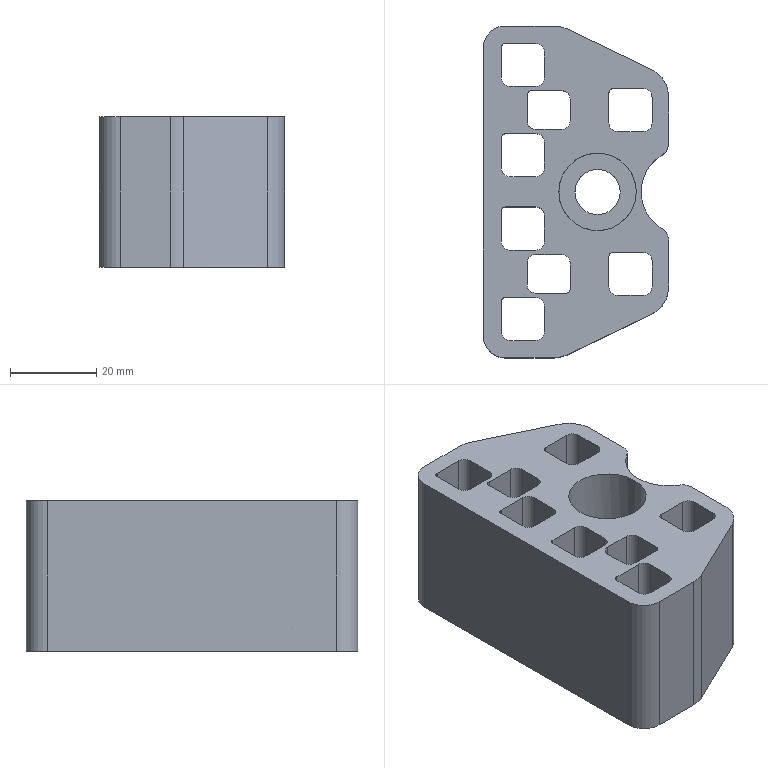Part | NX | features DIE-90 2 | 1 solid | 116 faces | box 43 x 77 x 35 mm | volume 69181 mm3 | plane 57 | cylinder 57 | spline 2 | commonest cylinder face diameters 4 x24 6 x16 2 x8 14 x4 10 x2 10.506 x1